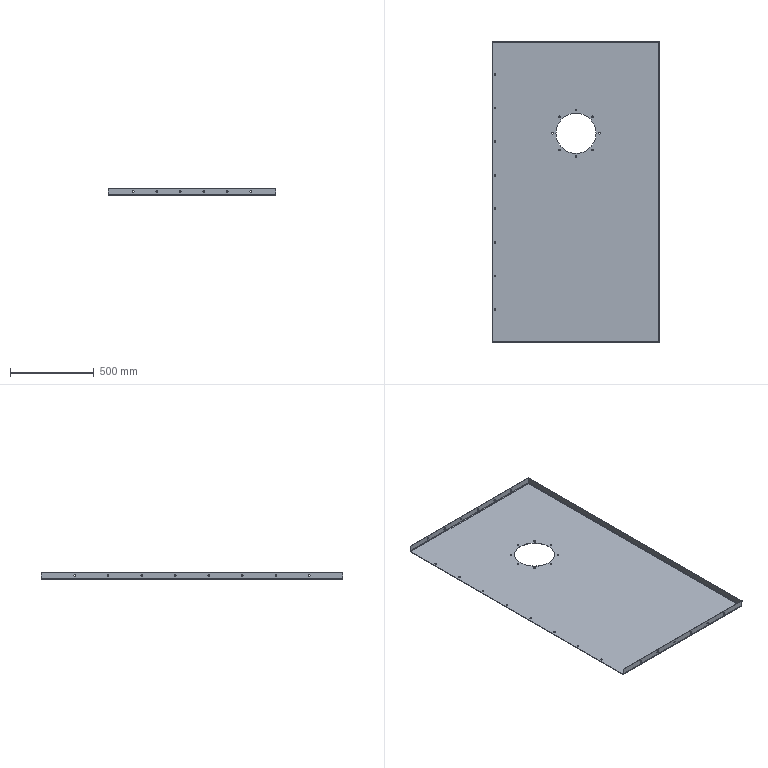Part | SolidWorks | features ICE 4, CirPattern 1, CornerFeat 1, EdgeFlange 1, FlatPattern 1, RefAxis 1, SMBaseFlange 1, SheetMetal 1 | 1 solid | 104 faces | box 1000 x 1800 x 40 mm | volume 5654846 mm3 | cylinder 80 | plane 20 | spline 4 | commonest cylinder face diameters 10 x72 6 x3 12 x3 240 x2